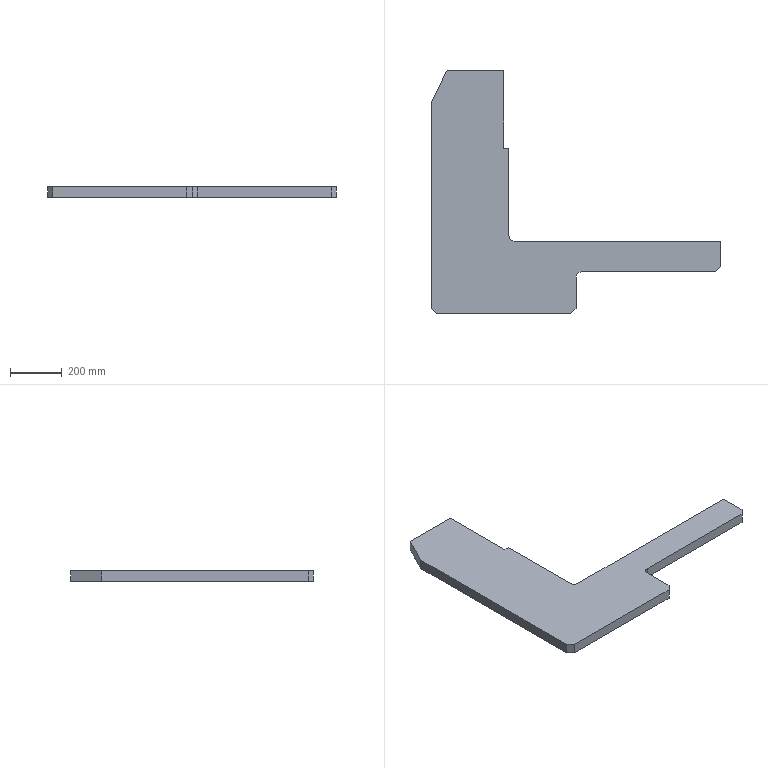Part | SolidWorks | features Chamfer 1, Extrusion 1, Fillet 1 | 1 solid | 18 faces | box 1120 x 940 x 40 mm | volume 16478867 mm3 | plane 16 | cylinder 2 | commonest cylinder face diameters 40 x2
STEP:
#1=CARTESIAN_POINT('',(-41.631,-67.27,0.));
#2=VERTEX_POINT('',#1);
#3=CARTESIAN_POINT('',(478.369,-67.27,0.));
#4=VERTEX_POINT('',#3);
#5=CARTESIAN_POINT('',(-61.631,-67.27,0.));
#6=DIRECTION('',(1.,0.,0.));
#7=VECTOR('',#6,1000.);
#8=LINE('',#5,#7);
#9=EDGE_CURVE('',#2,#4,#8,.T.);
#10=ORIENTED_EDGE('',*,*,#9,.T.);
#11=CARTESIAN_POINT('',(478.369,-67.27,40.));
#12=VERTEX_POINT('',#11);
#13=CARTESIAN_POINT('',(478.369,-67.27,40.));
#14=DIRECTION('',(0.,0.,1.));
#15=VECTOR('',#14,1000.);
#16=LINE('',#13,#15);
#17=EDGE_CURVE('',#4,#12,#16,.T.);
#18=ORIENTED_EDGE('',*,*,#17,.T.);
#19=CARTESIAN_POINT('',(-41.631,-67.27,40.));
#20=VERTEX_POINT('',#19);
#21=CARTESIAN_POINT('',(-61.631,-67.27,40.));
#22=DIRECTION('',(1.,0.,0.));
#23=VECTOR('',#22,1000.);
#24=LINE('',#21,#23);
#25=EDGE_CURVE('',#20,#12,#24,.T.);
#26=ORIENTED_EDGE('',*,*,#25,.F.);
#27=CARTESIAN_POINT('',(-41.631,-67.27,40.));
#28=DIRECTION('',(0.,0.,-1.));
#29=VECTOR('',#28,1000.);
#30=LINE('',#27,#29);
#31=EDGE_CURVE('',#20,#2,#30,.T.);
#32=ORIENTED_EDGE('',*,*,#31,.T.);
#33=EDGE_LOOP('',(#10,#18,#26,#32));
#34=FACE_OUTER_BOUND('',#33,.T.);
#35=CARTESIAN_POINT('',(-61.631,-67.27,40.));
#36=DIRECTION('',(0.,1.,0.));
#37=DIRECTION('',(0.,0.,1.));
#38=AXIS2_PLACEMENT_3D('',#35,#36,#37);
#39=PLANE('',#38);
#40=ADVANCED_FACE('',(#34),#39,.F.);
#41=CARTESIAN_POINT('',(498.369,-47.27,0.));
#42=VERTEX_POINT('',#41);
#43=CARTESIAN_POINT('',(498.369,72.73,0.));
#44=VERTEX_POINT('',#43);
#45=CARTESIAN_POINT('',(498.369,-67.27,0.));
#46=DIRECTION('',(0.,1.,0.));
#47=VECTOR('',#46,1000.);
#48=LINE('',#45,#47);
#49=EDGE_CURVE('',#42,#44,#48,.T.);
#50=ORIENTED_EDGE('',*,*,#49,.T.);
#51=CARTESIAN_POINT('',(498.369,72.73,40.));
#52=VERTEX_POINT('',#51);
#53=CARTESIAN_POINT('',(498.369,72.73,40.));
#54=DIRECTION('',(0.,0.,1.));
#55=VECTOR('',#54,1000.);
#56=LINE('',#53,#55);
#57=EDGE_CURVE('',#44,#52,#56,.T.);
#58=ORIENTED_EDGE('',*,*,#57,.T.);
#59=CARTESIAN_POINT('',(498.369,-47.27,40.));
#60=VERTEX_POINT('',#59);
#61=CARTESIAN_POINT('',(498.369,-67.27,40.));
#62=DIRECTION('',(0.,1.,0.));
#63=VECTOR('',#62,1000.);
#64=LINE('',#61,#63);
#65=EDGE_CURVE('',#60,#52,#64,.T.);
#66=ORIENTED_EDGE('',*,*,#65,.F.);
#67=CARTESIAN_POINT('',(498.369,-47.27,40.));
#68=DIRECTION('',(0.,0.,-1.));
#69=VECTOR('',#68,1000.);
#70=LINE('',#67,#69);
#71=EDGE_CURVE('',#60,#42,#70,.T.);
#72=ORIENTED_EDGE('',*,*,#71,.T.);
#73=EDGE_LOOP('',(#50,#58,#66,#72));
#74=FACE_OUTER_BOUND('',#73,.T.);
#75=CARTESIAN_POINT('',(498.369,-67.27,40.));
#76=DIRECTION('',(-1.,0.,0.));
#77=DIRECTION('',(0.,0.,1.));
#78=AXIS2_PLACEMENT_3D('',#75,#76,#77);
#79=PLANE('',#78);
#80=ADVANCED_FACE('',(#74),#79,.F.);
#81=CARTESIAN_POINT('',(518.369,92.73,40.));
#82=VERTEX_POINT('',#81);
#83=CARTESIAN_POINT('',(1038.369,92.73,40.));
#84=VERTEX_POINT('',#83);
#85=CARTESIAN_POINT('',(498.369,92.73,40.));
#86=DIRECTION('',(1.,0.,0.));
#87=VECTOR('',#86,1000.);
#88=LINE('',#85,#87);
#89=EDGE_CURVE('',#82,#84,#88,.T.);
#90=ORIENTED_EDGE('',*,*,#89,.F.);
#91=CARTESIAN_POINT('',(518.369,92.73,0.));
#92=VERTEX_POINT('',#91);
#93=CARTESIAN_POINT('',(518.369,92.73,0.));
#94=DIRECTION('',(0.,0.,-1.));
#95=VECTOR('',#94,1000.);
#96=LINE('',#93,#95);
#97=EDGE_CURVE('',#82,#92,#96,.T.);
#98=ORIENTED_EDGE('',*,*,#97,.T.);
#99=CARTESIAN_POINT('',(1038.369,92.73,0.));
#100=VERTEX_POINT('',#99);
#101=CARTESIAN_POINT('',(498.369,92.73,0.));
#102=DIRECTION('',(1.,0.,0.));
#103=VECTOR('',#102,1000.);
#104=LINE('',#101,#103);
#105=EDGE_CURVE('',#92,#100,#104,.T.);
#106=ORIENTED_EDGE('',*,*,#105,.T.);
#107=CARTESIAN_POINT('',(1038.369,92.73,40.));
#108=DIRECTION('',(0.,0.,1.));
#109=VECTOR('',#108,1000.);
#110=LINE('',#107,#109);
#111=EDGE_CURVE('',#100,#84,#110,.T.);
#112=ORIENTED_EDGE('',*,*,#111,.T.);
#113=EDGE_LOOP('',(#90,#98,#106,#112));
#114=FACE_OUTER_BOUND('',#113,.T.);
#115=CARTESIAN_POINT('',(498.369,92.73,40.));
#116=DIRECTION('',(0.,1.,0.));
#117=DIRECTION('',(0.,0.,1.));
#118=AXIS2_PLACEMENT_3D('',#115,#116,#117);
#119=PLANE('',#118);
#120=ADVANCED_FACE('',(#114),#119,.F.);
#121=CARTESIAN_POINT('',(1058.369,112.73,40.));
#122=VERTEX_POINT('',#121);
#123=CARTESIAN_POINT('',(1058.369,212.73,40.));
#124=VERTEX_POINT('',#123);
#125=CARTESIAN_POINT('',(1058.369,92.73,40.));
#126=DIRECTION('',(0.,1.,0.));
#127=VECTOR('',#126,1000.);
#128=LINE('',#125,#127);
#129=EDGE_CURVE('',#122,#124,#128,.T.);
#130=ORIENTED_EDGE('',*,*,#129,.F.);
#131=CARTESIAN_POINT('',(1058.369,112.73,0.));
#132=VERTEX_POINT('',#131);
#133=CARTESIAN_POINT('',(1058.369,112.73,40.));
#134=DIRECTION('',(0.,0.,-1.));
#135=VECTOR('',#134,1000.);
#136=LINE('',#133,#135);
#137=EDGE_CURVE('',#122,#132,#136,.T.);
#138=ORIENTED_EDGE('',*,*,#137,.T.);
#139=CARTESIAN_POINT('',(1058.369,212.73,0.));
#140=VERTEX_POINT('',#139);
#141=CARTESIAN_POINT('',(1058.369,92.73,0.));
#142=DIRECTION('',(0.,1.,0.));
#143=VECTOR('',#142,1000.);
#144=LINE('',#141,#143);
#145=EDGE_CURVE('',#132,#140,#144,.T.);
#146=ORIENTED_EDGE('',*,*,#145,.T.);
#147=CARTESIAN_POINT('',(1058.369,212.73,40.));
#148=DIRECTION('',(0.,0.,-1.));
#149=VECTOR('',#148,1000.);
#150=LINE('',#147,#149);
#151=EDGE_CURVE('',#124,#140,#150,.T.);
#152=ORIENTED_EDGE('',*,*,#151,.F.);
#153=EDGE_LOOP('',(#130,#138,#146,#152));
#154=FACE_OUTER_BOUND('',#153,.T.);
#155=CARTESIAN_POINT('',(1058.369,92.73,40.));
#156=DIRECTION('',(-1.,0.,0.));
#157=DIRECTION('',(0.,0.,1.));
#158=AXIS2_PLACEMENT_3D('',#155,#156,#157);
#159=PLANE('',#158);
#160=ADVANCED_FACE('',(#154),#159,.F.);
#161=CARTESIAN_POINT('',(258.369,212.73,0.));
#162=VERTEX_POINT('',#161);
#163=CARTESIAN_POINT('',(1058.369,212.73,0.));
#164=DIRECTION('',(-1.,0.,0.));
#165=VECTOR('',#164,1000.);
#166=LINE('',#163,#165);
#167=EDGE_CURVE('',#140,#162,#166,.T.);
#168=ORIENTED_EDGE('',*,*,#167,.T.);
#169=CARTESIAN_POINT('',(258.369,212.73,40.));
#170=VERTEX_POINT('',#169);
#171=CARTESIAN_POINT('',(258.369,212.73,40.));
#172=DIRECTION('',(0.,0.,1.));
#173=VECTOR('',#172,1000.);
#174=LINE('',#171,#173);
#175=EDGE_CURVE('',#162,#170,#174,.T.);
#176=ORIENTED_EDGE('',*,*,#175,.T.);
#177=CARTESIAN_POINT('',(1058.369,212.73,40.));
#178=DIRECTION('',(-1.,0.,0.));
#179=VECTOR('',#178,1000.);
#180=LINE('',#177,#179);
#181=EDGE_CURVE('',#124,#170,#180,.T.);
#182=ORIENTED_EDGE('',*,*,#181,.F.);
#183=ORIENTED_EDGE('',*,*,#151,.T.);
#184=EDGE_LOOP('',(#168,#176,#182,#183));
#185=FACE_OUTER_BOUND('',#184,.T.);
#186=CARTESIAN_POINT('',(1058.369,212.73,40.));
#187=DIRECTION('',(0.,-1.,0.));
#188=DIRECTION('',(1.,0.,0.));
#189=AXIS2_PLACEMENT_3D('',#186,#187,#188);
#190=PLANE('',#189);
#191=ADVANCED_FACE('',(#185),#190,.F.);
#192=CARTESIAN_POINT('',(238.369,232.73,40.));
#193=VERTEX_POINT('',#192);
#194=CARTESIAN_POINT('',(238.369,572.73,40.));
#195=VERTEX_POINT('',#194);
#196=CARTESIAN_POINT('',(238.369,212.73,40.));
#197=DIRECTION('',(0.,1.,0.));
#198=VECTOR('',#197,1000.);
#199=LINE('',#196,#198);
#200=EDGE_CURVE('',#193,#195,#199,.T.);
#201=ORIENTED_EDGE('',*,*,#200,.F.);
#202=CARTESIAN_POINT('',(238.369,232.73,0.));
#203=VERTEX_POINT('',#202);
#204=CARTESIAN_POINT('',(238.369,232.73,0.));
#205=DIRECTION('',(0.,0.,-1.));
#206=VECTOR('',#205,1000.);
#207=LINE('',#204,#206);
#208=EDGE_CURVE('',#193,#203,#207,.T.);
#209=ORIENTED_EDGE('',*,*,#208,.T.);
#210=CARTESIAN_POINT('',(238.369,572.73,0.));
#211=VERTEX_POINT('',#210);
#212=CARTESIAN_POINT('',(238.369,212.73,0.));
#213=DIRECTION('',(0.,1.,0.));
#214=VECTOR('',#213,1000.);
#215=LINE('',#212,#214);
#216=EDGE_CURVE('',#203,#211,#215,.T.);
#217=ORIENTED_EDGE('',*,*,#216,.T.);
#218=CARTESIAN_POINT('',(238.369,572.73,40.));
#219=DIRECTION('',(0.,0.,-1.));
#220=VECTOR('',#219,1000.);
#221=LINE('',#218,#220);
#222=EDGE_CURVE('',#195,#211,#221,.T.);
#223=ORIENTED_EDGE('',*,*,#222,.F.);
#224=EDGE_LOOP('',(#201,#209,#217,#223));
#225=FACE_OUTER_BOUND('',#224,.T.);
#226=CARTESIAN_POINT('',(238.369,212.73,40.));
#227=DIRECTION('',(-1.,0.,0.));
#228=DIRECTION('',(0.,0.,1.));
#229=AXIS2_PLACEMENT_3D('',#226,#227,#228);
#230=PLANE('',#229);
#231=ADVANCED_FACE('',(#225),#230,.F.);
#232=CARTESIAN_POINT('',(218.369,572.73,0.));
#233=VERTEX_POINT('',#232);
#234=CARTESIAN_POINT('',(238.369,572.73,0.));
#235=DIRECTION('',(-1.,0.,0.));
#236=VECTOR('',#235,1000.);
#237=LINE('',#234,#236);
#238=EDGE_CURVE('',#211,#233,#237,.T.);
#239=ORIENTED_EDGE('',*,*,#238,.T.);
#240=CARTESIAN_POINT('',(218.369,572.73,40.));
#241=VERTEX_POINT('',#240);
#242=CARTESIAN_POINT('',(218.369,572.73,40.));
#243=DIRECTION('',(0.,0.,-1.));
#244=VECTOR('',#243,1000.);
#245=LINE('',#242,#244);
#246=EDGE_CURVE('',#241,#233,#245,.T.);
#247=ORIENTED_EDGE('',*,*,#246,.F.);
#248=CARTESIAN_POINT('',(238.369,572.73,40.));
#249=DIRECTION('',(-1.,0.,0.));
#250=VECTOR('',#249,1000.);
#251=LINE('',#248,#250);
#252=EDGE_CURVE('',#195,#241,#251,.T.);
#253=ORIENTED_EDGE('',*,*,#252,.F.);
#254=ORIENTED_EDGE('',*,*,#222,.T.);
#255=EDGE_LOOP('',(#239,#247,#253,#254));
#256=FACE_OUTER_BOUND('',#255,.T.);
#257=CARTESIAN_POINT('',(238.369,572.73,40.));
#258=DIRECTION('',(0.,-1.,0.));
#259=DIRECTION('',(0.,0.,-1.));
#260=AXIS2_PLACEMENT_3D('',#257,#258,#259);
#261=PLANE('',#260);
#262=ADVANCED_FACE('',(#256),#261,.F.);
#263=CARTESIAN_POINT('',(218.369,872.73,0.));
#264=VERTEX_POINT('',#263);
#265=CARTESIAN_POINT('',(218.369,572.73,0.));
#266=DIRECTION('',(0.,1.,0.));
#267=VECTOR('',#266,1000.);
#268=LINE('',#265,#267);
#269=EDGE_CURVE('',#233,#264,#268,.T.);
#270=ORIENTED_EDGE('',*,*,#269,.T.);
#271=CARTESIAN_POINT('',(218.369,872.73,40.));
#272=VERTEX_POINT('',#271);
#273=CARTESIAN_POINT('',(218.369,872.73,40.));
#274=DIRECTION('',(0.,0.,-1.));
#275=VECTOR('',#274,1000.);
#276=LINE('',#273,#275);
#277=EDGE_CURVE('',#272,#264,#276,.T.);
#278=ORIENTED_EDGE('',*,*,#277,.F.);
#279=CARTESIAN_POINT('',(218.369,572.73,40.));
#280=DIRECTION('',(0.,1.,0.));
#281=VECTOR('',#280,1000.);
#282=LINE('',#279,#281);
#283=EDGE_CURVE('',#241,#272,#282,.T.);
#284=ORIENTED_EDGE('',*,*,#283,.F.);
#285=ORIENTED_EDGE('',*,*,#246,.T.);
#286=EDGE_LOOP('',(#270,#278,#284,#285));
#287=FACE_OUTER_BOUND('',#286,.T.);
#288=CARTESIAN_POINT('',(218.369,572.73,40.));
#289=DIRECTION('',(-1.,0.,0.));
#290=DIRECTION('',(0.,0.,1.));
#291=AXIS2_PLACEMENT_3D('',#288,#289,#290);
#292=PLANE('',#291);
#293=ADVANCED_FACE('',(#287),#292,.F.);
#294=CARTESIAN_POINT('',(-1.631,872.73,0.));
#295=VERTEX_POINT('',#294);
#296=CARTESIAN_POINT('',(218.369,872.73,0.));
#297=DIRECTION('',(-1.,0.,0.));
#298=VECTOR('',#297,1000.);
#299=LINE('',#296,#298);
#300=EDGE_CURVE('',#264,#295,#299,.T.);
#301=ORIENTED_EDGE('',*,*,#300,.T.);
#302=CARTESIAN_POINT('',(-1.631,872.73,40.));
#303=VERTEX_POINT('',#302);
#304=CARTESIAN_POINT('',(-1.631,872.73,40.));
#305=DIRECTION('',(0.,0.,-1.));
#306=VECTOR('',#305,1000.);
#307=LINE('',#304,#306);
#308=EDGE_CURVE('',#303,#295,#307,.T.);
#309=ORIENTED_EDGE('',*,*,#308,.F.);
#310=CARTESIAN_POINT('',(218.369,872.73,40.));
#311=DIRECTION('',(-1.,0.,0.));
#312=VECTOR('',#311,1000.);
#313=LINE('',#310,#312);
#314=EDGE_CURVE('',#272,#303,#313,.T.);
#315=ORIENTED_EDGE('',*,*,#314,.F.);
#316=ORIENTED_EDGE('',*,*,#277,.T.);
#317=EDGE_LOOP('',(#301,#309,#315,#316));
#318=FACE_OUTER_BOUND('',#317,.T.);
#319=CARTESIAN_POINT('',(218.369,872.73,40.));
#320=DIRECTION('',(0.,-1.,0.));
#321=DIRECTION('',(0.,0.,-1.));
#322=AXIS2_PLACEMENT_3D('',#319,#320,#321);
#323=PLANE('',#322);
#324=ADVANCED_FACE('',(#318),#323,.F.);
#325=CARTESIAN_POINT('',(-61.631,752.73,0.));
#326=VERTEX_POINT('',#325);
#327=CARTESIAN_POINT('',(-61.631,752.73,0.));
#328=DIRECTION('',(-0.4472,-0.8944,0.));
#329=VECTOR('',#328,1000.);
#330=LINE('',#327,#329);
#331=EDGE_CURVE('',#295,#326,#330,.T.);
#332=ORIENTED_EDGE('',*,*,#331,.T.);
#333=CARTESIAN_POINT('',(-61.631,752.73,40.));
#334=VERTEX_POINT('',#333);
#335=CARTESIAN_POINT('',(-61.631,752.73,40.));
#336=DIRECTION('',(0.,0.,-1.));
#337=VECTOR('',#336,1000.);
#338=LINE('',#335,#337);
#339=EDGE_CURVE('',#334,#326,#338,.T.);
#340=ORIENTED_EDGE('',*,*,#339,.F.);
#341=CARTESIAN_POINT('',(-61.631,752.73,40.));
#342=DIRECTION('',(-0.4472,-0.8944,0.));
#343=VECTOR('',#342,1000.);
#344=LINE('',#341,#343);
#345=EDGE_CURVE('',#303,#334,#344,.T.);
#346=ORIENTED_EDGE('',*,*,#345,.F.);
#347=ORIENTED_EDGE('',*,*,#308,.T.);
#348=EDGE_LOOP('',(#332,#340,#346,#347));
#349=FACE_OUTER_BOUND('',#348,.T.);
#350=CARTESIAN_POINT('',(-61.631,752.73,40.));
#351=DIRECTION('',(0.8944,-0.4472,0.));
#352=DIRECTION('',(0.4472,0.8944,0.));
#353=AXIS2_PLACEMENT_3D('',#350,#351,#352);
#354=PLANE('',#353);
#355=ADVANCED_FACE('',(#349),#354,.F.);
#356=CARTESIAN_POINT('',(-61.631,-47.27,0.));
#357=VERTEX_POINT('',#356);
#358=CARTESIAN_POINT('',(-61.631,752.73,0.));
#359=DIRECTION('',(0.,-1.,0.));
#360=VECTOR('',#359,1000.);
#361=LINE('',#358,#360);
#362=EDGE_CURVE('',#326,#357,#361,.T.);
#363=ORIENTED_EDGE('',*,*,#362,.T.);
#364=CARTESIAN_POINT('',(-61.631,-47.27,40.));
#365=VERTEX_POINT('',#364);
#366=CARTESIAN_POINT('',(-61.631,-47.27,40.));
#367=DIRECTION('',(0.,0.,1.));
#368=VECTOR('',#367,1000.);
#369=LINE('',#366,#368);
#370=EDGE_CURVE('',#357,#365,#369,.T.);
#371=ORIENTED_EDGE('',*,*,#370,.T.);
#372=CARTESIAN_POINT('',(-61.631,752.73,40.));
#373=DIRECTION('',(0.,-1.,0.));
#374=VECTOR('',#373,1000.);
#375=LINE('',#372,#374);
#376=EDGE_CURVE('',#334,#365,#375,.T.);
#377=ORIENTED_EDGE('',*,*,#376,.F.);
#378=ORIENTED_EDGE('',*,*,#339,.T.);
#379=EDGE_LOOP('',(#363,#371,#377,#378));
#380=FACE_OUTER_BOUND('',#379,.T.);
#381=CARTESIAN_POINT('',(-61.631,752.73,40.));
#382=DIRECTION('',(1.,0.,0.));
#383=DIRECTION('',(0.,1.,0.));
#384=AXIS2_PLACEMENT_3D('',#381,#382,#383);
#385=PLANE('',#384);
#386=ADVANCED_FACE('',(#380),#385,.F.);
#387=ORIENTED_EDGE('',*,*,#65,.T.);
#388=CARTESIAN_POINT('',(518.369,72.73,40.));
#389=DIRECTION('',(0.,0.,-1.));
#390=DIRECTION('',(1.,0.,0.));
#391=AXIS2_PLACEMENT_3D('',#388,#389,#390);
#392=CIRCLE('',#391,20.);
#393=EDGE_CURVE('',#52,#82,#392,.T.);
#394=ORIENTED_EDGE('',*,*,#393,.T.);
#395=ORIENTED_EDGE('',*,*,#89,.T.);
#396=CARTESIAN_POINT('',(472.82,-472.82,40.));
#397=DIRECTION('',(0.7071,0.7071,0.));
#398=VECTOR('',#397,1000.);
#399=LINE('',#396,#398);
#400=EDGE_CURVE('',#84,#122,#399,.T.);
#401=ORIENTED_EDGE('',*,*,#400,.T.);
#402=ORIENTED_EDGE('',*,*,#129,.T.);
#403=ORIENTED_EDGE('',*,*,#181,.T.);
#404=CARTESIAN_POINT('',(258.369,232.73,40.));
#405=DIRECTION('',(0.,0.,-1.));
#406=DIRECTION('',(1.,0.,0.));
#407=AXIS2_PLACEMENT_3D('',#404,#405,#406);
#408=CIRCLE('',#407,20.);
#409=EDGE_CURVE('',#170,#193,#408,.T.);
#410=ORIENTED_EDGE('',*,*,#409,.T.);
#411=ORIENTED_EDGE('',*,*,#200,.T.);
#412=ORIENTED_EDGE('',*,*,#252,.T.);
#413=ORIENTED_EDGE('',*,*,#283,.T.);
#414=ORIENTED_EDGE('',*,*,#314,.T.);
#415=ORIENTED_EDGE('',*,*,#345,.T.);
#416=ORIENTED_EDGE('',*,*,#376,.T.);
#417=CARTESIAN_POINT('',(-54.451,-54.451,40.));
#418=DIRECTION('',(0.7071,-0.7071,0.));
#419=VECTOR('',#418,1000.);
#420=LINE('',#417,#419);
#421=EDGE_CURVE('',#365,#20,#420,.T.);
#422=ORIENTED_EDGE('',*,*,#421,.T.);
#423=ORIENTED_EDGE('',*,*,#25,.T.);
#424=CARTESIAN_POINT('',(272.82,-272.82,40.));
#425=DIRECTION('',(0.7071,0.7071,0.));
#426=VECTOR('',#425,1000.);
#427=LINE('',#424,#426);
#428=EDGE_CURVE('',#12,#60,#427,.T.);
#429=ORIENTED_EDGE('',*,*,#428,.T.);
#430=EDGE_LOOP('',(#387,#394,#395,#401,#402,#403,#410,#411,#412,#413,#414,#415,#416,#422,#423,#429));
#431=FACE_OUTER_BOUND('',#430,.T.);
#432=CARTESIAN_POINT('',(0.,0.,40.));
#433=DIRECTION('',(0.,0.,1.));
#434=DIRECTION('',(1.,0.,0.));
#435=AXIS2_PLACEMENT_3D('',#432,#433,#434);
#436=PLANE('',#435);
#437=ADVANCED_FACE('',(#431),#436,.T.);
#438=ORIENTED_EDGE('',*,*,#145,.F.);
#439=CARTESIAN_POINT('',(1058.369,112.73,0.));
#440=DIRECTION('',(-0.7071,-0.7071,0.));
#441=VECTOR('',#440,1000.);
#442=LINE('',#439,#441);
#443=EDGE_CURVE('',#132,#100,#442,.T.);
#444=ORIENTED_EDGE('',*,*,#443,.T.);
#445=ORIENTED_EDGE('',*,*,#105,.F.);
#446=CARTESIAN_POINT('',(518.369,72.73,0.));
#447=DIRECTION('',(0.,0.,1.));
#448=DIRECTION('',(1.,0.,0.));
#449=AXIS2_PLACEMENT_3D('',#446,#447,#448);
#450=CIRCLE('',#449,20.);
#451=EDGE_CURVE('',#92,#44,#450,.T.);
#452=ORIENTED_EDGE('',*,*,#451,.T.);
#453=ORIENTED_EDGE('',*,*,#49,.F.);
#454=CARTESIAN_POINT('',(498.369,-47.27,0.));
#455=DIRECTION('',(-0.7071,-0.7071,0.));
#456=VECTOR('',#455,1000.);
#457=LINE('',#454,#456);
#458=EDGE_CURVE('',#42,#4,#457,.T.);
#459=ORIENTED_EDGE('',*,*,#458,.T.);
#460=ORIENTED_EDGE('',*,*,#9,.F.);
#461=CARTESIAN_POINT('',(-41.631,-67.27,0.));
#462=DIRECTION('',(-0.7071,0.7071,0.));
#463=VECTOR('',#462,1000.);
#464=LINE('',#461,#463);
#465=EDGE_CURVE('',#2,#357,#464,.T.);
#466=ORIENTED_EDGE('',*,*,#465,.T.);
#467=ORIENTED_EDGE('',*,*,#362,.F.);
#468=ORIENTED_EDGE('',*,*,#331,.F.);
#469=ORIENTED_EDGE('',*,*,#300,.F.);
#470=ORIENTED_EDGE('',*,*,#269,.F.);
#471=ORIENTED_EDGE('',*,*,#238,.F.);
#472=ORIENTED_EDGE('',*,*,#216,.F.);
#473=CARTESIAN_POINT('',(258.369,232.73,0.));
#474=DIRECTION('',(0.,0.,1.));
#475=DIRECTION('',(1.,0.,0.));
#476=AXIS2_PLACEMENT_3D('',#473,#474,#475);
#477=CIRCLE('',#476,20.);
#478=EDGE_CURVE('',#203,#162,#477,.T.);
#479=ORIENTED_EDGE('',*,*,#478,.T.);
#480=ORIENTED_EDGE('',*,*,#167,.F.);
#481=EDGE_LOOP('',(#438,#444,#445,#452,#453,#459,#460,#466,#467,#468,#469,#470,#471,#472,#479,#480));
#482=FACE_OUTER_BOUND('',#481,.T.);
#483=CARTESIAN_POINT('',(0.,0.,0.));
#484=DIRECTION('',(0.,0.,1.));
#485=DIRECTION('',(1.,0.,0.));
#486=AXIS2_PLACEMENT_3D('',#483,#484,#485);
#487=PLANE('',#486);
#488=ADVANCED_FACE('',(#482),#487,.F.);
#489=ORIENTED_EDGE('',*,*,#400,.F.);
#490=ORIENTED_EDGE('',*,*,#111,.F.);
#491=ORIENTED_EDGE('',*,*,#443,.F.);
#492=ORIENTED_EDGE('',*,*,#137,.F.);
#493=EDGE_LOOP('',(#489,#490,#491,#492));
#494=FACE_OUTER_BOUND('',#493,.T.);
#495=CARTESIAN_POINT('',(1058.369,112.73,40.));
#496=DIRECTION('',(-0.7071,0.7071,0.));
#497=DIRECTION('',(0.,0.,-1.));
#498=AXIS2_PLACEMENT_3D('',#495,#496,#497);
#499=PLANE('',#498);
#500=ADVANCED_FACE('',(#494),#499,.F.);
#501=ORIENTED_EDGE('',*,*,#428,.F.);
#502=ORIENTED_EDGE('',*,*,#17,.F.);
#503=ORIENTED_EDGE('',*,*,#458,.F.);
#504=ORIENTED_EDGE('',*,*,#71,.F.);
#505=EDGE_LOOP('',(#501,#502,#503,#504));
#506=FACE_OUTER_BOUND('',#505,.T.);
#507=CARTESIAN_POINT('',(498.369,-47.27,40.));
#508=DIRECTION('',(-0.7071,0.7071,0.));
#509=DIRECTION('',(0.,0.,-1.));
#510=AXIS2_PLACEMENT_3D('',#507,#508,#509);
#511=PLANE('',#510);
#512=ADVANCED_FACE('',(#506),#511,.F.);
#513=ORIENTED_EDGE('',*,*,#421,.F.);
#514=ORIENTED_EDGE('',*,*,#370,.F.);
#515=ORIENTED_EDGE('',*,*,#465,.F.);
#516=ORIENTED_EDGE('',*,*,#31,.F.);
#517=EDGE_LOOP('',(#513,#514,#515,#516));
#518=FACE_OUTER_BOUND('',#517,.T.);
#519=CARTESIAN_POINT('',(-41.631,-67.27,40.));
#520=DIRECTION('',(0.7071,0.7071,0.));
#521=DIRECTION('',(0.,0.,-1.));
#522=AXIS2_PLACEMENT_3D('',#519,#520,#521);
#523=PLANE('',#522);
#524=ADVANCED_FACE('',(#518),#523,.F.);
#525=ORIENTED_EDGE('',*,*,#393,.F.);
#526=ORIENTED_EDGE('',*,*,#57,.F.);
#527=ORIENTED_EDGE('',*,*,#451,.F.);
#528=ORIENTED_EDGE('',*,*,#97,.F.);
#529=EDGE_LOOP('',(#525,#526,#527,#528));
#530=FACE_OUTER_BOUND('',#529,.T.);
#531=CARTESIAN_POINT('',(518.369,72.73,40.));
#532=DIRECTION('',(0.,0.,1.));
#533=DIRECTION('',(1.,0.,0.));
#534=AXIS2_PLACEMENT_3D('',#531,#532,#533);
#535=CYLINDRICAL_SURFACE('',#534,20.);
#536=ADVANCED_FACE('',(#530),#535,.F.);
#537=ORIENTED_EDGE('',*,*,#409,.F.);
#538=ORIENTED_EDGE('',*,*,#175,.F.);
#539=ORIENTED_EDGE('',*,*,#478,.F.);
#540=ORIENTED_EDGE('',*,*,#208,.F.);
#541=EDGE_LOOP('',(#537,#538,#539,#540));
#542=FACE_OUTER_BOUND('',#541,.T.);
#543=CARTESIAN_POINT('',(258.369,232.73,40.));
#544=DIRECTION('',(0.,0.,1.));
#545=DIRECTION('',(1.,0.,0.));
#546=AXIS2_PLACEMENT_3D('',#543,#544,#545);
#547=CYLINDRICAL_SURFACE('',#546,20.);
#548=ADVANCED_FACE('',(#542),#547,.F.);
#549=CLOSED_SHELL('',(#40,#80,#120,#160,#191,#231,#262,#293,#324,#355,#386,#437,#488,#500,#512,#524,#536,#548));
#550=MANIFOLD_SOLID_BREP('',#549);
#551=CARTESIAN_POINT('',(0.,0.,0.));
#552=DIRECTION('',(0.,0.,1.));
#553=DIRECTION('',(1.,0.,0.));
#554=AXIS2_PLACEMENT_3D('',#551,#552,#553);
#555=(LENGTH_UNIT()NAMED_UNIT(*)SI_UNIT(.MILLI.,.METRE.));
#556=UNCERTAINTY_MEASURE_WITH_UNIT(LENGTH_MEASURE(0.00001),#555,'','');
#557=(NAMED_UNIT(*)PLANE_ANGLE_UNIT()SI_UNIT($,.RADIAN.));
#558=(NAMED_UNIT(*)SI_UNIT($,.STERADIAN.)SOLID_ANGLE_UNIT());
#559=(GEOMETRIC_REPRESENTATION_CONTEXT(3)GLOBAL_UNCERTAINTY_ASSIGNED_CONTEXT((#556))GLOBAL_UNIT_ASSIGNED_CONTEXT((#555,#557,#558))REPRESENTATION_CONTEXT('',''));
#560=ADVANCED_BREP_SHAPE_REPRESENTATION('',(#550,#554),#559);